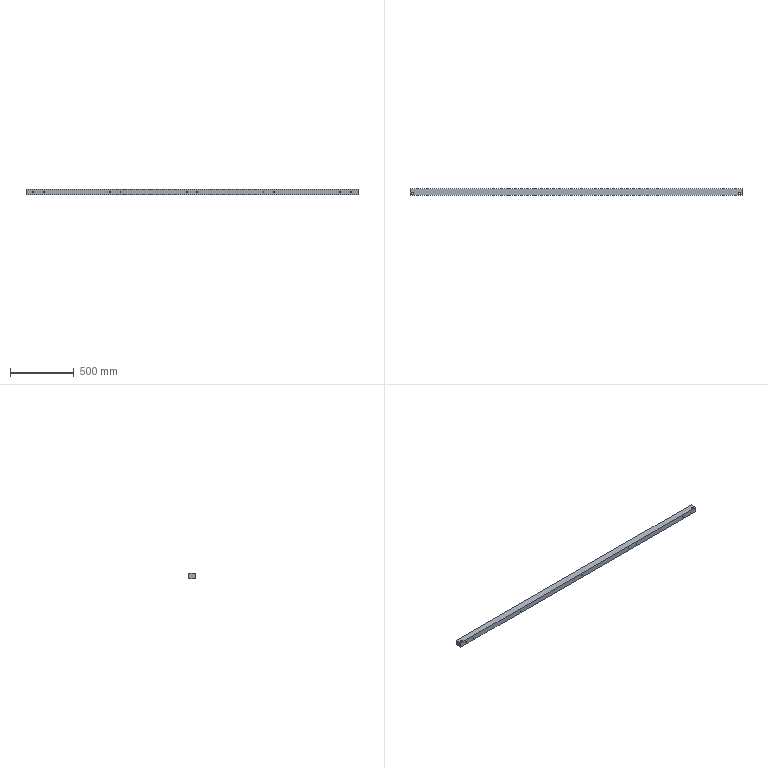Part | SolidWorks | features ICE 2, Extrusion 1 | 1 solid | 30 faces | box 2596 x 50 x 40 mm | volume 5166098 mm3 | cylinder 24 | plane 6 | commonest cylinder face diameters 5 x20 16 x4
STEP:
#1=CARTESIAN_POINT('',(1286.,15.,20.));
#2=VERTEX_POINT('',#1);
#3=CARTESIAN_POINT('',(1270.,15.,20.));
#4=VERTEX_POINT('',#3);
#5=CARTESIAN_POINT('',(1278.,15.,20.));
#6=DIRECTION('',(0.,0.,-1.));
#7=DIRECTION('',(-1.,0.,0.));
#8=AXIS2_PLACEMENT_3D('',#5,#6,#7);
#9=CIRCLE('',#8,8.);
#10=EDGE_CURVE('',#2,#4,#9,.T.);
#11=ORIENTED_EDGE('',*,*,#10,.F.);
#12=CARTESIAN_POINT('',(1286.,15.,-20.));
#13=VERTEX_POINT('',#12);
#14=CARTESIAN_POINT('',(1286.,15.,30.));
#15=DIRECTION('',(0.,0.,-1.));
#16=VECTOR('',#15,1000.);
#17=LINE('',#14,#16);
#18=EDGE_CURVE('',#2,#13,#17,.T.);
#19=ORIENTED_EDGE('',*,*,#18,.T.);
#20=CARTESIAN_POINT('',(1270.,15.,-20.));
#21=VERTEX_POINT('',#20);
#22=CARTESIAN_POINT('',(1278.,15.,-20.));
#23=DIRECTION('',(0.,0.,-1.));
#24=DIRECTION('',(-1.,0.,0.));
#25=AXIS2_PLACEMENT_3D('',#22,#23,#24);
#26=CIRCLE('',#25,8.);
#27=EDGE_CURVE('',#13,#21,#26,.T.);
#28=ORIENTED_EDGE('',*,*,#27,.T.);
#29=CARTESIAN_POINT('',(1270.,15.,30.));
#30=DIRECTION('',(0.,0.,-1.));
#31=VECTOR('',#30,1000.);
#32=LINE('',#29,#31);
#33=EDGE_CURVE('',#4,#21,#32,.T.);
#34=ORIENTED_EDGE('',*,*,#33,.F.);
#35=EDGE_LOOP('',(#11,#19,#28,#34));
#36=FACE_OUTER_BOUND('',#35,.T.);
#37=CARTESIAN_POINT('',(1278.,15.,30.));
#38=DIRECTION('',(0.,0.,-1.));
#39=DIRECTION('',(-1.,0.,0.));
#40=AXIS2_PLACEMENT_3D('',#37,#38,#39);
#41=CYLINDRICAL_SURFACE('',#40,8.);
#42=ADVANCED_FACE('',(#36),#41,.F.);
#43=CARTESIAN_POINT('',(-1270.,15.,20.));
#44=VERTEX_POINT('',#43);
#45=CARTESIAN_POINT('',(-1286.,15.,20.));
#46=VERTEX_POINT('',#45);
#47=CARTESIAN_POINT('',(-1278.,15.,20.));
#48=DIRECTION('',(0.,0.,-1.));
#49=DIRECTION('',(-1.,0.,0.));
#50=AXIS2_PLACEMENT_3D('',#47,#48,#49);
#51=CIRCLE('',#50,8.);
#52=EDGE_CURVE('',#44,#46,#51,.T.);
#53=ORIENTED_EDGE('',*,*,#52,.F.);
#54=CARTESIAN_POINT('',(-1270.,15.,-20.));
#55=VERTEX_POINT('',#54);
#56=CARTESIAN_POINT('',(-1270.,15.,30.));
#57=DIRECTION('',(0.,0.,-1.));
#58=VECTOR('',#57,1000.);
#59=LINE('',#56,#58);
#60=EDGE_CURVE('',#44,#55,#59,.T.);
#61=ORIENTED_EDGE('',*,*,#60,.T.);
#62=CARTESIAN_POINT('',(-1286.,15.,-20.));
#63=VERTEX_POINT('',#62);
#64=CARTESIAN_POINT('',(-1278.,15.,-20.));
#65=DIRECTION('',(0.,0.,-1.));
#66=DIRECTION('',(1.,0.,0.));
#67=AXIS2_PLACEMENT_3D('',#64,#65,#66);
#68=CIRCLE('',#67,8.);
#69=EDGE_CURVE('',#55,#63,#68,.T.);
#70=ORIENTED_EDGE('',*,*,#69,.T.);
#71=CARTESIAN_POINT('',(-1286.,15.,30.));
#72=DIRECTION('',(0.,0.,-1.));
#73=VECTOR('',#72,1000.);
#74=LINE('',#71,#73);
#75=EDGE_CURVE('',#46,#63,#74,.T.);
#76=ORIENTED_EDGE('',*,*,#75,.F.);
#77=EDGE_LOOP('',(#53,#61,#70,#76));
#78=FACE_OUTER_BOUND('',#77,.T.);
#79=CARTESIAN_POINT('',(-1278.,15.,30.));
#80=DIRECTION('',(0.,0.,-1.));
#81=DIRECTION('',(-1.,0.,0.));
#82=AXIS2_PLACEMENT_3D('',#79,#80,#81);
#83=CYLINDRICAL_SURFACE('',#82,8.);
#84=ADVANCED_FACE('',(#78),#83,.F.);
#85=CARTESIAN_POINT('',(1241.5,50.,2.5));
#86=VERTEX_POINT('',#85);
#87=CARTESIAN_POINT('',(1241.5,50.,-2.5));
#88=VERTEX_POINT('',#87);
#89=CARTESIAN_POINT('',(1241.5,50.,0.));
#90=DIRECTION('',(0.,-1.,0.));
#91=DIRECTION('',(0.,0.,-1.));
#92=AXIS2_PLACEMENT_3D('',#89,#90,#91);
#93=CIRCLE('',#92,2.5);
#94=EDGE_CURVE('',#86,#88,#93,.T.);
#95=ORIENTED_EDGE('',*,*,#94,.F.);
#96=CARTESIAN_POINT('',(1241.5,0.,2.5));
#97=VERTEX_POINT('',#96);
#98=CARTESIAN_POINT('',(1241.5,50.,2.5));
#99=DIRECTION('',(0.,-1.,0.));
#100=VECTOR('',#99,1000.);
#101=LINE('',#98,#100);
#102=EDGE_CURVE('',#86,#97,#101,.T.);
#103=ORIENTED_EDGE('',*,*,#102,.T.);
#104=CARTESIAN_POINT('',(1241.5,0.,-2.5));
#105=VERTEX_POINT('',#104);
#106=CARTESIAN_POINT('',(1241.5,0.,0.));
#107=DIRECTION('',(0.,-1.,0.));
#108=DIRECTION('',(0.,0.,-1.));
#109=AXIS2_PLACEMENT_3D('',#106,#107,#108);
#110=CIRCLE('',#109,2.5);
#111=EDGE_CURVE('',#97,#105,#110,.T.);
#112=ORIENTED_EDGE('',*,*,#111,.T.);
#113=CARTESIAN_POINT('',(1241.5,50.,-2.5));
#114=DIRECTION('',(0.,-1.,0.));
#115=VECTOR('',#114,1000.);
#116=LINE('',#113,#115);
#117=EDGE_CURVE('',#88,#105,#116,.T.);
#118=ORIENTED_EDGE('',*,*,#117,.F.);
#119=EDGE_LOOP('',(#95,#103,#112,#118));
#120=FACE_OUTER_BOUND('',#119,.T.);
#121=CARTESIAN_POINT('',(1241.5,50.,0.));
#122=DIRECTION('',(0.,-1.,0.));
#123=DIRECTION('',(0.,0.,-1.));
#124=AXIS2_PLACEMENT_3D('',#121,#122,#123);
#125=CYLINDRICAL_SURFACE('',#124,2.5);
#126=ADVANCED_FACE('',(#120),#125,.F.);
#127=CARTESIAN_POINT('',(1158.5,50.,2.5));
#128=VERTEX_POINT('',#127);
#129=CARTESIAN_POINT('',(1158.5,50.,-2.5));
#130=VERTEX_POINT('',#129);
#131=CARTESIAN_POINT('',(1158.5,50.,0.));
#132=DIRECTION('',(0.,-1.,0.));
#133=DIRECTION('',(0.,0.,-1.));
#134=AXIS2_PLACEMENT_3D('',#131,#132,#133);
#135=CIRCLE('',#134,2.5);
#136=EDGE_CURVE('',#128,#130,#135,.T.);
#137=ORIENTED_EDGE('',*,*,#136,.F.);
#138=CARTESIAN_POINT('',(1158.5,0.,2.5));
#139=VERTEX_POINT('',#138);
#140=CARTESIAN_POINT('',(1158.5,50.,2.5));
#141=DIRECTION('',(0.,-1.,0.));
#142=VECTOR('',#141,1000.);
#143=LINE('',#140,#142);
#144=EDGE_CURVE('',#128,#139,#143,.T.);
#145=ORIENTED_EDGE('',*,*,#144,.T.);
#146=CARTESIAN_POINT('',(1158.5,0.,-2.5));
#147=VERTEX_POINT('',#146);
#148=CARTESIAN_POINT('',(1158.5,0.,0.));
#149=DIRECTION('',(0.,-1.,0.));
#150=DIRECTION('',(0.,0.,-1.));
#151=AXIS2_PLACEMENT_3D('',#148,#149,#150);
#152=CIRCLE('',#151,2.5);
#153=EDGE_CURVE('',#139,#147,#152,.T.);
#154=ORIENTED_EDGE('',*,*,#153,.T.);
#155=CARTESIAN_POINT('',(1158.5,50.,-2.5));
#156=DIRECTION('',(0.,-1.,0.));
#157=VECTOR('',#156,1000.);
#158=LINE('',#155,#157);
#159=EDGE_CURVE('',#130,#147,#158,.T.);
#160=ORIENTED_EDGE('',*,*,#159,.F.);
#161=EDGE_LOOP('',(#137,#145,#154,#160));
#162=FACE_OUTER_BOUND('',#161,.T.);
#163=CARTESIAN_POINT('',(1158.5,50.,0.));
#164=DIRECTION('',(0.,-1.,0.));
#165=DIRECTION('',(0.,0.,-1.));
#166=AXIS2_PLACEMENT_3D('',#163,#164,#165);
#167=CYLINDRICAL_SURFACE('',#166,2.5);
#168=ADVANCED_FACE('',(#162),#167,.F.);
#169=CARTESIAN_POINT('',(641.5,50.,2.5));
#170=VERTEX_POINT('',#169);
#171=CARTESIAN_POINT('',(641.5,50.,-2.5));
#172=VERTEX_POINT('',#171);
#173=CARTESIAN_POINT('',(641.5,50.,0.));
#174=DIRECTION('',(0.,-1.,0.));
#175=DIRECTION('',(0.,0.,-1.));
#176=AXIS2_PLACEMENT_3D('',#173,#174,#175);
#177=CIRCLE('',#176,2.5);
#178=EDGE_CURVE('',#170,#172,#177,.T.);
#179=ORIENTED_EDGE('',*,*,#178,.F.);
#180=CARTESIAN_POINT('',(641.5,0.,2.5));
#181=VERTEX_POINT('',#180);
#182=CARTESIAN_POINT('',(641.5,50.,2.5));
#183=DIRECTION('',(0.,-1.,0.));
#184=VECTOR('',#183,1000.);
#185=LINE('',#182,#184);
#186=EDGE_CURVE('',#170,#181,#185,.T.);
#187=ORIENTED_EDGE('',*,*,#186,.T.);
#188=CARTESIAN_POINT('',(641.5,0.,-2.5));
#189=VERTEX_POINT('',#188);
#190=CARTESIAN_POINT('',(641.5,0.,0.));
#191=DIRECTION('',(0.,-1.,0.));
#192=DIRECTION('',(0.,0.,-1.));
#193=AXIS2_PLACEMENT_3D('',#190,#191,#192);
#194=CIRCLE('',#193,2.5);
#195=EDGE_CURVE('',#181,#189,#194,.T.);
#196=ORIENTED_EDGE('',*,*,#195,.T.);
#197=CARTESIAN_POINT('',(641.5,50.,-2.5));
#198=DIRECTION('',(0.,-1.,0.));
#199=VECTOR('',#198,1000.);
#200=LINE('',#197,#199);
#201=EDGE_CURVE('',#172,#189,#200,.T.);
#202=ORIENTED_EDGE('',*,*,#201,.F.);
#203=EDGE_LOOP('',(#179,#187,#196,#202));
#204=FACE_OUTER_BOUND('',#203,.T.);
#205=CARTESIAN_POINT('',(641.5,50.,0.));
#206=DIRECTION('',(0.,-1.,0.));
#207=DIRECTION('',(0.,0.,-1.));
#208=AXIS2_PLACEMENT_3D('',#205,#206,#207);
#209=CYLINDRICAL_SURFACE('',#208,2.5);
#210=ADVANCED_FACE('',(#204),#209,.F.);
#211=CARTESIAN_POINT('',(558.5,50.,2.5));
#212=VERTEX_POINT('',#211);
#213=CARTESIAN_POINT('',(558.5,50.,-2.5));
#214=VERTEX_POINT('',#213);
#215=CARTESIAN_POINT('',(558.5,50.,0.));
#216=DIRECTION('',(0.,-1.,0.));
#217=DIRECTION('',(0.,0.,-1.));
#218=AXIS2_PLACEMENT_3D('',#215,#216,#217);
#219=CIRCLE('',#218,2.5);
#220=EDGE_CURVE('',#212,#214,#219,.T.);
#221=ORIENTED_EDGE('',*,*,#220,.F.);
#222=CARTESIAN_POINT('',(558.5,0.,2.5));
#223=VERTEX_POINT('',#222);
#224=CARTESIAN_POINT('',(558.5,50.,2.5));
#225=DIRECTION('',(0.,-1.,0.));
#226=VECTOR('',#225,1000.);
#227=LINE('',#224,#226);
#228=EDGE_CURVE('',#212,#223,#227,.T.);
#229=ORIENTED_EDGE('',*,*,#228,.T.);
#230=CARTESIAN_POINT('',(558.5,0.,-2.5));
#231=VERTEX_POINT('',#230);
#232=CARTESIAN_POINT('',(558.5,0.,0.));
#233=DIRECTION('',(0.,-1.,0.));
#234=DIRECTION('',(0.,0.,-1.));
#235=AXIS2_PLACEMENT_3D('',#232,#233,#234);
#236=CIRCLE('',#235,2.5);
#237=EDGE_CURVE('',#223,#231,#236,.T.);
#238=ORIENTED_EDGE('',*,*,#237,.T.);
#239=CARTESIAN_POINT('',(558.5,50.,-2.5));
#240=DIRECTION('',(0.,-1.,0.));
#241=VECTOR('',#240,1000.);
#242=LINE('',#239,#241);
#243=EDGE_CURVE('',#214,#231,#242,.T.);
#244=ORIENTED_EDGE('',*,*,#243,.F.);
#245=EDGE_LOOP('',(#221,#229,#238,#244));
#246=FACE_OUTER_BOUND('',#245,.T.);
#247=CARTESIAN_POINT('',(558.5,50.,0.));
#248=DIRECTION('',(0.,-1.,0.));
#249=DIRECTION('',(0.,0.,-1.));
#250=AXIS2_PLACEMENT_3D('',#247,#248,#249);
#251=CYLINDRICAL_SURFACE('',#250,2.5);
#252=ADVANCED_FACE('',(#246),#251,.F.);
#253=CARTESIAN_POINT('',(41.5,50.,2.5));
#254=VERTEX_POINT('',#253);
#255=CARTESIAN_POINT('',(41.5,50.,-2.5));
#256=VERTEX_POINT('',#255);
#257=CARTESIAN_POINT('',(41.5,50.,0.));
#258=DIRECTION('',(0.,-1.,0.));
#259=DIRECTION('',(0.,0.,-1.));
#260=AXIS2_PLACEMENT_3D('',#257,#258,#259);
#261=CIRCLE('',#260,2.5);
#262=EDGE_CURVE('',#254,#256,#261,.T.);
#263=ORIENTED_EDGE('',*,*,#262,.F.);
#264=CARTESIAN_POINT('',(41.5,0.,2.5));
#265=VERTEX_POINT('',#264);
#266=CARTESIAN_POINT('',(41.5,50.,2.5));
#267=DIRECTION('',(0.,-1.,0.));
#268=VECTOR('',#267,1000.);
#269=LINE('',#266,#268);
#270=EDGE_CURVE('',#254,#265,#269,.T.);
#271=ORIENTED_EDGE('',*,*,#270,.T.);
#272=CARTESIAN_POINT('',(41.5,0.,-2.5));
#273=VERTEX_POINT('',#272);
#274=CARTESIAN_POINT('',(41.5,0.,0.));
#275=DIRECTION('',(0.,-1.,0.));
#276=DIRECTION('',(0.,0.,-1.));
#277=AXIS2_PLACEMENT_3D('',#274,#275,#276);
#278=CIRCLE('',#277,2.5);
#279=EDGE_CURVE('',#265,#273,#278,.T.);
#280=ORIENTED_EDGE('',*,*,#279,.T.);
#281=CARTESIAN_POINT('',(41.5,50.,-2.5));
#282=DIRECTION('',(0.,-1.,0.));
#283=VECTOR('',#282,1000.);
#284=LINE('',#281,#283);
#285=EDGE_CURVE('',#256,#273,#284,.T.);
#286=ORIENTED_EDGE('',*,*,#285,.F.);
#287=EDGE_LOOP('',(#263,#271,#280,#286));
#288=FACE_OUTER_BOUND('',#287,.T.);
#289=CARTESIAN_POINT('',(41.5,50.,0.));
#290=DIRECTION('',(0.,-1.,0.));
#291=DIRECTION('',(0.,0.,-1.));
#292=AXIS2_PLACEMENT_3D('',#289,#290,#291);
#293=CYLINDRICAL_SURFACE('',#292,2.5);
#294=ADVANCED_FACE('',(#288),#293,.F.);
#295=CARTESIAN_POINT('',(-41.5,50.,2.5));
#296=VERTEX_POINT('',#295);
#297=CARTESIAN_POINT('',(-41.5,50.,-2.5));
#298=VERTEX_POINT('',#297);
#299=CARTESIAN_POINT('',(-41.5,50.,0.));
#300=DIRECTION('',(0.,-1.,0.));
#301=DIRECTION('',(0.,0.,1.));
#302=AXIS2_PLACEMENT_3D('',#299,#300,#301);
#303=CIRCLE('',#302,2.5);
#304=EDGE_CURVE('',#296,#298,#303,.T.);
#305=ORIENTED_EDGE('',*,*,#304,.F.);
#306=CARTESIAN_POINT('',(-41.5,0.,2.5));
#307=VERTEX_POINT('',#306);
#308=CARTESIAN_POINT('',(-41.5,50.,2.5));
#309=DIRECTION('',(0.,-1.,0.));
#310=VECTOR('',#309,1000.);
#311=LINE('',#308,#310);
#312=EDGE_CURVE('',#296,#307,#311,.T.);
#313=ORIENTED_EDGE('',*,*,#312,.T.);
#314=CARTESIAN_POINT('',(-41.5,0.,-2.5));
#315=VERTEX_POINT('',#314);
#316=CARTESIAN_POINT('',(-41.5,0.,0.));
#317=DIRECTION('',(0.,-1.,0.));
#318=DIRECTION('',(0.,0.,1.));
#319=AXIS2_PLACEMENT_3D('',#316,#317,#318);
#320=CIRCLE('',#319,2.5);
#321=EDGE_CURVE('',#307,#315,#320,.T.);
#322=ORIENTED_EDGE('',*,*,#321,.T.);
#323=CARTESIAN_POINT('',(-41.5,50.,-2.5));
#324=DIRECTION('',(0.,-1.,0.));
#325=VECTOR('',#324,1000.);
#326=LINE('',#323,#325);
#327=EDGE_CURVE('',#298,#315,#326,.T.);
#328=ORIENTED_EDGE('',*,*,#327,.F.);
#329=EDGE_LOOP('',(#305,#313,#322,#328));
#330=FACE_OUTER_BOUND('',#329,.T.);
#331=CARTESIAN_POINT('',(-41.5,50.,0.));
#332=DIRECTION('',(0.,-1.,0.));
#333=DIRECTION('',(0.,0.,-1.));
#334=AXIS2_PLACEMENT_3D('',#331,#332,#333);
#335=CYLINDRICAL_SURFACE('',#334,2.5);
#336=ADVANCED_FACE('',(#330),#335,.F.);
#337=CARTESIAN_POINT('',(-558.5,50.,2.5));
#338=VERTEX_POINT('',#337);
#339=CARTESIAN_POINT('',(-558.5,50.,-2.5));
#340=VERTEX_POINT('',#339);
#341=CARTESIAN_POINT('',(-558.5,50.,0.));
#342=DIRECTION('',(0.,-1.,0.));
#343=DIRECTION('',(0.,0.,1.));
#344=AXIS2_PLACEMENT_3D('',#341,#342,#343);
#345=CIRCLE('',#344,2.5);
#346=EDGE_CURVE('',#338,#340,#345,.T.);
#347=ORIENTED_EDGE('',*,*,#346,.F.);
#348=CARTESIAN_POINT('',(-558.5,0.,2.5));
#349=VERTEX_POINT('',#348);
#350=CARTESIAN_POINT('',(-558.5,50.,2.5));
#351=DIRECTION('',(0.,-1.,0.));
#352=VECTOR('',#351,1000.);
#353=LINE('',#350,#352);
#354=EDGE_CURVE('',#338,#349,#353,.T.);
#355=ORIENTED_EDGE('',*,*,#354,.T.);
#356=CARTESIAN_POINT('',(-558.5,0.,-2.5));
#357=VERTEX_POINT('',#356);
#358=CARTESIAN_POINT('',(-558.5,0.,0.));
#359=DIRECTION('',(0.,-1.,0.));
#360=DIRECTION('',(0.,0.,1.));
#361=AXIS2_PLACEMENT_3D('',#358,#359,#360);
#362=CIRCLE('',#361,2.5);
#363=EDGE_CURVE('',#349,#357,#362,.T.);
#364=ORIENTED_EDGE('',*,*,#363,.T.);
#365=CARTESIAN_POINT('',(-558.5,50.,-2.5));
#366=DIRECTION('',(0.,-1.,0.));
#367=VECTOR('',#366,1000.);
#368=LINE('',#365,#367);
#369=EDGE_CURVE('',#340,#357,#368,.T.);
#370=ORIENTED_EDGE('',*,*,#369,.F.);
#371=EDGE_LOOP('',(#347,#355,#364,#370));
#372=FACE_OUTER_BOUND('',#371,.T.);
#373=CARTESIAN_POINT('',(-558.5,50.,0.));
#374=DIRECTION('',(0.,-1.,0.));
#375=DIRECTION('',(0.,0.,-1.));
#376=AXIS2_PLACEMENT_3D('',#373,#374,#375);
#377=CYLINDRICAL_SURFACE('',#376,2.5);
#378=ADVANCED_FACE('',(#372),#377,.F.);
#379=CARTESIAN_POINT('',(-641.5,50.,2.5));
#380=VERTEX_POINT('',#379);
#381=CARTESIAN_POINT('',(-641.5,50.,-2.5));
#382=VERTEX_POINT('',#381);
#383=CARTESIAN_POINT('',(-641.5,50.,0.));
#384=DIRECTION('',(0.,-1.,0.));
#385=DIRECTION('',(0.,0.,1.));
#386=AXIS2_PLACEMENT_3D('',#383,#384,#385);
#387=CIRCLE('',#386,2.5);
#388=EDGE_CURVE('',#380,#382,#387,.T.);
#389=ORIENTED_EDGE('',*,*,#388,.F.);
#390=CARTESIAN_POINT('',(-641.5,0.,2.5));
#391=VERTEX_POINT('',#390);
#392=CARTESIAN_POINT('',(-641.5,50.,2.5));
#393=DIRECTION('',(0.,-1.,0.));
#394=VECTOR('',#393,1000.);
#395=LINE('',#392,#394);
#396=EDGE_CURVE('',#380,#391,#395,.T.);
#397=ORIENTED_EDGE('',*,*,#396,.T.);
#398=CARTESIAN_POINT('',(-641.5,0.,-2.5));
#399=VERTEX_POINT('',#398);
#400=CARTESIAN_POINT('',(-641.5,0.,0.));
#401=DIRECTION('',(0.,-1.,0.));
#402=DIRECTION('',(0.,0.,1.));
#403=AXIS2_PLACEMENT_3D('',#400,#401,#402);
#404=CIRCLE('',#403,2.5);
#405=EDGE_CURVE('',#391,#399,#404,.T.);
#406=ORIENTED_EDGE('',*,*,#405,.T.);
#407=CARTESIAN_POINT('',(-641.5,50.,-2.5));
#408=DIRECTION('',(0.,-1.,0.));
#409=VECTOR('',#408,1000.);
#410=LINE('',#407,#409);
#411=EDGE_CURVE('',#382,#399,#410,.T.);
#412=ORIENTED_EDGE('',*,*,#411,.F.);
#413=EDGE_LOOP('',(#389,#397,#406,#412));
#414=FACE_OUTER_BOUND('',#413,.T.);
#415=CARTESIAN_POINT('',(-641.5,50.,0.));
#416=DIRECTION('',(0.,-1.,0.));
#417=DIRECTION('',(0.,0.,-1.));
#418=AXIS2_PLACEMENT_3D('',#415,#416,#417);
#419=CYLINDRICAL_SURFACE('',#418,2.5);
#420=ADVANCED_FACE('',(#414),#419,.F.);
#421=CARTESIAN_POINT('',(-1158.5,50.,2.5));
#422=VERTEX_POINT('',#421);
#423=CARTESIAN_POINT('',(-1158.5,50.,-2.5));
#424=VERTEX_POINT('',#423);
#425=CARTESIAN_POINT('',(-1158.5,50.,0.));
#426=DIRECTION('',(0.,-1.,0.));
#427=DIRECTION('',(0.,0.,1.));
#428=AXIS2_PLACEMENT_3D('',#425,#426,#427);
#429=CIRCLE('',#428,2.5);
#430=EDGE_CURVE('',#422,#424,#429,.T.);
#431=ORIENTED_EDGE('',*,*,#430,.F.);
#432=CARTESIAN_POINT('',(-1158.5,0.,2.5));
#433=VERTEX_POINT('',#432);
#434=CARTESIAN_POINT('',(-1158.5,50.,2.5));
#435=DIRECTION('',(0.,-1.,0.));
#436=VECTOR('',#435,1000.);
#437=LINE('',#434,#436);
#438=EDGE_CURVE('',#422,#433,#437,.T.);
#439=ORIENTED_EDGE('',*,*,#438,.T.);
#440=CARTESIAN_POINT('',(-1158.5,0.,-2.5));
#441=VERTEX_POINT('',#440);
#442=CARTESIAN_POINT('',(-1158.5,0.,0.));
#443=DIRECTION('',(0.,-1.,0.));
#444=DIRECTION('',(0.,0.,1.));
#445=AXIS2_PLACEMENT_3D('',#442,#443,#444);
#446=CIRCLE('',#445,2.5);
#447=EDGE_CURVE('',#433,#441,#446,.T.);
#448=ORIENTED_EDGE('',*,*,#447,.T.);
#449=CARTESIAN_POINT('',(-1158.5,50.,-2.5));
#450=DIRECTION('',(0.,-1.,0.));
#451=VECTOR('',#450,1000.);
#452=LINE('',#449,#451);
#453=EDGE_CURVE('',#424,#441,#452,.T.);
#454=ORIENTED_EDGE('',*,*,#453,.F.);
#455=EDGE_LOOP('',(#431,#439,#448,#454));
#456=FACE_OUTER_BOUND('',#455,.T.);
#457=CARTESIAN_POINT('',(-1158.5,50.,0.));
#458=DIRECTION('',(0.,-1.,0.));
#459=DIRECTION('',(0.,0.,-1.));
#460=AXIS2_PLACEMENT_3D('',#457,#458,#459);
#461=CYLINDRICAL_SURFACE('',#460,2.5);
#462=ADVANCED_FACE('',(#456),#461,.F.);
#463=CARTESIAN_POINT('',(-1241.5,50.,2.5));
#464=VERTEX_POINT('',#463);
#465=CARTESIAN_POINT('',(-1241.5,50.,-2.5));
#466=VERTEX_POINT('',#465);
#467=CARTESIAN_POINT('',(-1241.5,50.,0.));
#468=DIRECTION('',(0.,-1.,0.));
#469=DIRECTION('',(0.,0.,1.));
#470=AXIS2_PLACEMENT_3D('',#467,#468,#469);
#471=CIRCLE('',#470,2.5);
#472=EDGE_CURVE('',#464,#466,#471,.T.);
#473=ORIENTED_EDGE('',*,*,#472,.F.);
#474=CARTESIAN_POINT('',(-1241.5,0.,2.5));
#475=VERTEX_POINT('',#474);
#476=CARTESIAN_POINT('',(-1241.5,50.,2.5));
#477=DIRECTION('',(0.,-1.,0.));
#478=VECTOR('',#477,1000.);
#479=LINE('',#476,#478);
#480=EDGE_CURVE('',#464,#475,#479,.T.);
#481=ORIENTED_EDGE('',*,*,#480,.T.);
#482=CARTESIAN_POINT('',(-1241.5,0.,-2.5));
#483=VERTEX_POINT('',#482);
#484=CARTESIAN_POINT('',(-1241.5,0.,0.));
#485=DIRECTION('',(0.,-1.,0.));
#486=DIRECTION('',(0.,0.,1.));
#487=AXIS2_PLACEMENT_3D('',#484,#485,#486);
#488=CIRCLE('',#487,2.5);
#489=EDGE_CURVE('',#475,#483,#488,.T.);
#490=ORIENTED_EDGE('',*,*,#489,.T.);
#491=CARTESIAN_POINT('',(-1241.5,50.,-2.5));
#492=DIRECTION('',(0.,-1.,0.));
#493=VECTOR('',#492,1000.);
#494=LINE('',#491,#493);
#495=EDGE_CURVE('',#466,#483,#494,.T.);
#496=ORIENTED_EDGE('',*,*,#495,.F.);
#497=EDGE_LOOP('',(#473,#481,#490,#496));
#498=FACE_OUTER_BOUND('',#497,.T.);
#499=CARTESIAN_POINT('',(-1241.5,50.,0.));
#500=DIRECTION('',(0.,-1.,0.));
#501=DIRECTION('',(0.,0.,-1.));
#502=AXIS2_PLACEMENT_3D('',#499,#500,#501);
#503=CYLINDRICAL_SURFACE('',#502,2.5);
#504=ADVANCED_FACE('',(#498),#503,.F.);
#505=CARTESIAN_POINT('',(1298.,0.,20.));
#506=VERTEX_POINT('',#505);
#507=CARTESIAN_POINT('',(1298.,0.,-20.));
#508=VERTEX_POINT('',#507);
#509=CARTESIAN_POINT('',(1298.,0.,20.));
#510=DIRECTION('',(0.,0.,-1.));
#511=VECTOR('',#510,1000.);
#512=LINE('',#509,#511);
#513=EDGE_CURVE('',#506,#508,#512,.T.);
#514=ORIENTED_EDGE('',*,*,#513,.T.);
#515=CARTESIAN_POINT('',(1298.,50.,-20.));
#516=VERTEX_POINT('',#515);
#517=CARTESIAN_POINT('',(1298.,50.,-20.));
#518=DIRECTION('',(0.,-1.,0.));
#519=VECTOR('',#518,1000.);
#520=LINE('',#517,#519);
#521=EDGE_CURVE('',#516,#508,#520,.T.);
#522=ORIENTED_EDGE('',*,*,#521,.F.);
#523=CARTESIAN_POINT('',(1298.,50.,20.));
#524=VERTEX_POINT('',#523);
#525=CARTESIAN_POINT('',(1298.,50.,20.));
#526=DIRECTION('',(0.,0.,-1.));
#527=VECTOR('',#526,1000.);
#528=LINE('',#525,#527);
#529=EDGE_CURVE('',#524,#516,#528,.T.);
#530=ORIENTED_EDGE('',*,*,#529,.F.);
#531=CARTESIAN_POINT('',(1298.,50.,20.));
#532=DIRECTION('',(0.,-1.,0.));
#533=VECTOR('',#532,1000.);
#534=LINE('',#531,#533);
#535=EDGE_CURVE('',#524,#506,#534,.T.);
#536=ORIENTED_EDGE('',*,*,#535,.T.);
#537=EDGE_LOOP('',(#514,#522,#530,#536));
#538=FACE_OUTER_BOUND('',#537,.T.);
#539=CARTESIAN_POINT('',(1298.,50.,20.));
#540=DIRECTION('',(-1.,0.,0.));
#541=DIRECTION('',(0.,0.,1.));
#542=AXIS2_PLACEMENT_3D('',#539,#540,#541);
#543=PLANE('',#542);
#544=ADVANCED_FACE('',(#538),#543,.F.);
#545=CARTESIAN_POINT('',(1278.,15.,-20.));
#546=DIRECTION('',(0.,0.,-1.));
#547=DIRECTION('',(-1.,0.,0.));
#548=AXIS2_PLACEMENT_3D('',#545,#546,#547);
#549=CIRCLE('',#548,8.);
#550=EDGE_CURVE('',#21,#13,#549,.T.);
#551=ORIENTED_EDGE('',*,*,#550,.F.);
#552=ORIENTED_EDGE('',*,*,#27,.F.);
#553=EDGE_LOOP('',(#551,#552));
#554=FACE_BOUND('',#553,.T.);
#555=CARTESIAN_POINT('',(-1278.,15.,-20.));
#556=DIRECTION('',(0.,0.,-1.));
#557=DIRECTION('',(1.,0.,0.));
#558=AXIS2_PLACEMENT_3D('',#555,#556,#557);
#559=CIRCLE('',#558,8.);
#560=EDGE_CURVE('',#63,#55,#559,.T.);
#561=ORIENTED_EDGE('',*,*,#560,.F.);
#562=ORIENTED_EDGE('',*,*,#69,.F.);
#563=EDGE_LOOP('',(#561,#562));
#564=FACE_BOUND('',#563,.T.);
#565=CARTESIAN_POINT('',(-1298.,0.,-20.));
#566=VERTEX_POINT('',#565);
#567=CARTESIAN_POINT('',(-1298.,0.,-20.));
#568=DIRECTION('',(-1.,0.,0.));
#569=VECTOR('',#568,1000.);
#570=LINE('',#567,#569);
#571=EDGE_CURVE('',#508,#566,#570,.T.);
#572=ORIENTED_EDGE('',*,*,#571,.T.);
#573=CARTESIAN_POINT('',(-1298.,50.,-20.));
#574=VERTEX_POINT('',#573);
#575=CARTESIAN_POINT('',(-1298.,50.,-20.));
#576=DIRECTION('',(0.,-1.,0.));
#577=VECTOR('',#576,1000.);
#578=LINE('',#575,#577);
#579=EDGE_CURVE('',#574,#566,#578,.T.);
#580=ORIENTED_EDGE('',*,*,#579,.F.);
#581=CARTESIAN_POINT('',(-1298.,50.,-20.));
#582=DIRECTION('',(-1.,0.,0.));
#583=VECTOR('',#582,1000.);
#584=LINE('',#581,#583);
#585=EDGE_CURVE('',#516,#574,#584,.T.);
#586=ORIENTED_EDGE('',*,*,#585,.F.);
#587=ORIENTED_EDGE('',*,*,#521,.T.);
#588=EDGE_LOOP('',(#572,#580,#586,#587));
#589=FACE_OUTER_BOUND('',#588,.T.);
#590=CARTESIAN_POINT('',(-1298.,50.,-20.));
#591=DIRECTION('',(0.,0.,1.));
#592=DIRECTION('',(1.,0.,0.));
#593=AXIS2_PLACEMENT_3D('',#590,#591,#592);
#594=PLANE('',#593);
#595=ADVANCED_FACE('',(#554,#564,#589),#594,.F.);
#596=CARTESIAN_POINT('',(-1298.,0.,20.));
#597=VERTEX_POINT('',#596);
#598=CARTESIAN_POINT('',(-1298.,0.,20.));
#599=DIRECTION('',(0.,0.,1.));
#600=VECTOR('',#599,1000.);
#601=LINE('',#598,#600);
#602=EDGE_CURVE('',#566,#597,#601,.T.);
#603=ORIENTED_EDGE('',*,*,#602,.T.);
#604=CARTESIAN_POINT('',(-1298.,50.,20.));
#605=VERTEX_POINT('',#604);
#606=CARTESIAN_POINT('',(-1298.,50.,20.));
#607=DIRECTION('',(0.,-1.,0.));
#608=VECTOR('',#607,1000.);
#609=LINE('',#606,#608);
#610=EDGE_CURVE('',#605,#597,#609,.T.);
#611=ORIENTED_EDGE('',*,*,#610,.F.);
#612=CARTESIAN_POINT('',(-1298.,50.,20.));
#613=DIRECTION('',(0.,0.,1.));
#614=VECTOR('',#613,1000.);
#615=LINE('',#612,#614);
#616=EDGE_CURVE('',#574,#605,#615,.T.);
#617=ORIENTED_EDGE('',*,*,#616,.F.);
#618=ORIENTED_EDGE('',*,*,#579,.T.);
#619=EDGE_LOOP('',(#603,#611,#617,#618));
#620=FACE_OUTER_BOUND('',#619,.T.);
#621=CARTESIAN_POINT('',(-1298.,50.,20.));
#622=DIRECTION('',(1.,0.,0.));
#623=DIRECTION('',(0.,0.,-1.));
#624=AXIS2_PLACEMENT_3D('',#621,#622,#623);
#625=PLANE('',#624);
#626=ADVANCED_FACE('',(#620),#625,.F.);
#627=CARTESIAN_POINT('',(1278.,15.,20.));
#628=DIRECTION('',(0.,0.,-1.));
#629=DIRECTION('',(-1.,0.,0.));
#630=AXIS2_PLACEMENT_3D('',#627,#628,#629);
#631=CIRCLE('',#630,8.);
#632=EDGE_CURVE('',#4,#2,#631,.T.);
#633=ORIENTED_EDGE('',*,*,#632,.T.);
#634=ORIENTED_EDGE('',*,*,#10,.T.);
#635=EDGE_LOOP('',(#633,#634));
#636=FACE_BOUND('',#635,.T.);
#637=CARTESIAN_POINT('',(-1278.,15.,20.));
#638=DIRECTION('',(0.,0.,-1.));
#639=DIRECTION('',(-1.,0.,0.));
#640=AXIS2_PLACEMENT_3D('',#637,#638,#639);
#641=CIRCLE('',#640,8.);
#642=EDGE_CURVE('',#46,#44,#641,.T.);
#643=ORIENTED_EDGE('',*,*,#642,.T.);
#644=ORIENTED_EDGE('',*,*,#52,.T.);
#645=EDGE_LOOP('',(#643,#644));
#646=FACE_BOUND('',#645,.T.);
#647=CARTESIAN_POINT('',(-1298.,0.,20.));
#648=DIRECTION('',(1.,0.,0.));
#649=VECTOR('',#648,1000.);
#650=LINE('',#647,#649);
#651=EDGE_CURVE('',#597,#506,#650,.T.);
#652=ORIENTED_EDGE('',*,*,#651,.T.);
#653=ORIENTED_EDGE('',*,*,#535,.F.);
#654=CARTESIAN_POINT('',(-1298.,50.,20.));
#655=DIRECTION('',(1.,0.,0.));
#656=VECTOR('',#655,1000.);
#657=LINE('',#654,#656);
#658=EDGE_CURVE('',#605,#524,#657,.T.);
#659=ORIENTED_EDGE('',*,*,#658,.F.);
#660=ORIENTED_EDGE('',*,*,#610,.T.);
#661=EDGE_LOOP('',(#652,#653,#659,#660));
#662=FACE_OUTER_BOUND('',#661,.T.);
#663=CARTESIAN_POINT('',(-1298.,50.,20.));
#664=DIRECTION('',(0.,0.,-1.));
#665=DIRECTION('',(-1.,0.,0.));
#666=AXIS2_PLACEMENT_3D('',#663,#664,#665);
#667=PLANE('',#666);
#668=ADVANCED_FACE('',(#636,#646,#662),#667,.F.);
#669=CARTESIAN_POINT('',(1241.5,50.,0.));
#670=DIRECTION('',(0.,-1.,0.));
#671=DIRECTION('',(0.,0.,-1.));
#672=AXIS2_PLACEMENT_3D('',#669,#670,#671);
#673=CIRCLE('',#672,2.5);
#674=EDGE_CURVE('',#88,#86,#673,.T.);
#675=ORIENTED_EDGE('',*,*,#674,.T.);
#676=ORIENTED_EDGE('',*,*,#94,.T.);
#677=EDGE_LOOP('',(#675,#676));
#678=FACE_BOUND('',#677,.T.);
#679=CARTESIAN_POINT('',(1158.5,50.,0.));
#680=DIRECTION('',(0.,-1.,0.));
#681=DIRECTION('',(0.,0.,-1.));
#682=AXIS2_PLACEMENT_3D('',#679,#680,#681);
#683=CIRCLE('',#682,2.5);
#684=EDGE_CURVE('',#130,#128,#683,.T.);
#685=ORIENTED_EDGE('',*,*,#684,.T.);
#686=ORIENTED_EDGE('',*,*,#136,.T.);
#687=EDGE_LOOP('',(#685,#686));
#688=FACE_BOUND('',#687,.T.);
#689=CARTESIAN_POINT('',(641.5,50.,0.));
#690=DIRECTION('',(0.,-1.,0.));
#691=DIRECTION('',(0.,0.,-1.));
#692=AXIS2_PLACEMENT_3D('',#689,#690,#691);
#693=CIRCLE('',#692,2.5);
#694=EDGE_CURVE('',#172,#170,#693,.T.);
#695=ORIENTED_EDGE('',*,*,#694,.T.);
#696=ORIENTED_EDGE('',*,*,#178,.T.);
#697=EDGE_LOOP('',(#695,#696));
#698=FACE_BOUND('',#697,.T.);
#699=CARTESIAN_POINT('',(558.5,50.,0.));
#700=DIRECTION('',(0.,-1.,0.));
#701=DIRECTION('',(0.,0.,-1.));
#702=AXIS2_PLACEMENT_3D('',#699,#700,#701);
#703=CIRCLE('',#702,2.5);
#704=EDGE_CURVE('',#214,#212,#703,.T.);
#705=ORIENTED_EDGE('',*,*,#704,.T.);
#706=ORIENTED_EDGE('',*,*,#220,.T.);
#707=EDGE_LOOP('',(#705,#706));
#708=FACE_BOUND('',#707,.T.);
#709=CARTESIAN_POINT('',(41.5,50.,0.));
#710=DIRECTION('',(0.,-1.,0.));
#711=DIRECTION('',(0.,0.,-1.));
#712=AXIS2_PLACEMENT_3D('',#709,#710,#711);
#713=CIRCLE('',#712,2.5);
#714=EDGE_CURVE('',#256,#254,#713,.T.);
#715=ORIENTED_EDGE('',*,*,#714,.T.);
#716=ORIENTED_EDGE('',*,*,#262,.T.);
#717=EDGE_LOOP('',(#715,#716));
#718=FACE_BOUND('',#717,.T.);
#719=CARTESIAN_POINT('',(-41.5,50.,0.));
#720=DIRECTION('',(0.,-1.,0.));
#721=DIRECTION('',(0.,0.,1.));
#722=AXIS2_PLACEMENT_3D('',#719,#720,#721);
#723=CIRCLE('',#722,2.5);
#724=EDGE_CURVE('',#298,#296,#723,.T.);
#725=ORIENTED_EDGE('',*,*,#724,.T.);
#726=ORIENTED_EDGE('',*,*,#304,.T.);
#727=EDGE_LOOP('',(#725,#726));
#728=FACE_BOUND('',#727,.T.);
#729=CARTESIAN_POINT('',(-558.5,50.,0.));
#730=DIRECTION('',(0.,-1.,0.));
#731=DIRECTION('',(0.,0.,1.));
#732=AXIS2_PLACEMENT_3D('',#729,#730,#731);
#733=CIRCLE('',#732,2.5);
#734=EDGE_CURVE('',#340,#338,#733,.T.);
#735=ORIENTED_EDGE('',*,*,#734,.T.);
#736=ORIENTED_EDGE('',*,*,#346,.T.);
#737=EDGE_LOOP('',(#735,#736));
#738=FACE_BOUND('',#737,.T.);
#739=CARTESIAN_POINT('',(-641.5,50.,0.));
#740=DIRECTION('',(0.,-1.,0.));
#741=DIRECTION('',(0.,0.,1.));
#742=AXIS2_PLACEMENT_3D('',#739,#740,#741);
#743=CIRCLE('',#742,2.5);
#744=EDGE_CURVE('',#382,#380,#743,.T.);
#745=ORIENTED_EDGE('',*,*,#744,.T.);
#746=ORIENTED_EDGE('',*,*,#388,.T.);
#747=EDGE_LOOP('',(#745,#746));
#748=FACE_BOUND('',#747,.T.);
#749=CARTESIAN_POINT('',(-1158.5,50.,0.));
#750=DIRECTION('',(0.,-1.,0.));
#751=DIRECTION('',(0.,0.,1.));
#752=AXIS2_PLACEMENT_3D('',#749,#750,#751);
#753=CIRCLE('',#752,2.5);
#754=EDGE_CURVE('',#424,#422,#753,.T.);
#755=ORIENTED_EDGE('',*,*,#754,.T.);
#756=ORIENTED_EDGE('',*,*,#430,.T.);
#757=EDGE_LOOP('',(#755,#756));
#758=FACE_BOUND('',#757,.T.);
#759=CARTESIAN_POINT('',(-1241.5,50.,0.));
#760=DIRECTION('',(0.,-1.,0.));
#761=DIRECTION('',(0.,0.,1.));
#762=AXIS2_PLACEMENT_3D('',#759,#760,#761);
#763=CIRCLE('',#762,2.5);
#764=EDGE_CURVE('',#466,#464,#763,.T.);
#765=ORIENTED_EDGE('',*,*,#764,.T.);
#766=ORIENTED_EDGE('',*,*,#472,.T.);
#767=EDGE_LOOP('',(#765,#766));
#768=FACE_BOUND('',#767,.T.);
#769=ORIENTED_EDGE('',*,*,#529,.T.);
#770=ORIENTED_EDGE('',*,*,#585,.T.);
#771=ORIENTED_EDGE('',*,*,#616,.T.);
#772=ORIENTED_EDGE('',*,*,#658,.T.);
#773=EDGE_LOOP('',(#769,#770,#771,#772));
#774=FACE_OUTER_BOUND('',#773,.T.);
#775=CARTESIAN_POINT('',(0.,50.,0.));
#776=DIRECTION('',(0.,-1.,0.));
#777=DIRECTION('',(0.,0.,-1.));
#778=AXIS2_PLACEMENT_3D('',#775,#776,#777);
#779=PLANE('',#778);
#780=ADVANCED_FACE('',(#678,#688,#698,#708,#718,#728,#738,#748,#758,#768,#774),#779,.F.);
#781=CARTESIAN_POINT('',(1241.5,0.,0.));
#782=DIRECTION('',(0.,-1.,0.));
#783=DIRECTION('',(0.,0.,-1.));
#784=AXIS2_PLACEMENT_3D('',#781,#782,#783);
#785=CIRCLE('',#784,2.5);
#786=EDGE_CURVE('',#105,#97,#785,.T.);
#787=ORIENTED_EDGE('',*,*,#786,.F.);
#788=ORIENTED_EDGE('',*,*,#111,.F.);
#789=EDGE_LOOP('',(#787,#788));
#790=FACE_BOUND('',#789,.T.);
#791=CARTESIAN_POINT('',(1158.5,0.,0.));
#792=DIRECTION('',(0.,-1.,0.));
#793=DIRECTION('',(0.,0.,-1.));
#794=AXIS2_PLACEMENT_3D('',#791,#792,#793);
#795=CIRCLE('',#794,2.5);
#796=EDGE_CURVE('',#147,#139,#795,.T.);
#797=ORIENTED_EDGE('',*,*,#796,.F.);
#798=ORIENTED_EDGE('',*,*,#153,.F.);
#799=EDGE_LOOP('',(#797,#798));
#800=FACE_BOUND('',#799,.T.);
#801=CARTESIAN_POINT('',(641.5,0.,0.));
#802=DIRECTION('',(0.,-1.,0.));
#803=DIRECTION('',(0.,0.,-1.));
#804=AXIS2_PLACEMENT_3D('',#801,#802,#803);
#805=CIRCLE('',#804,2.5);
#806=EDGE_CURVE('',#189,#181,#805,.T.);
#807=ORIENTED_EDGE('',*,*,#806,.F.);
#808=ORIENTED_EDGE('',*,*,#195,.F.);
#809=EDGE_LOOP('',(#807,#808));
#810=FACE_BOUND('',#809,.T.);
#811=CARTESIAN_POINT('',(558.5,0.,0.));
#812=DIRECTION('',(0.,-1.,0.));
#813=DIRECTION('',(0.,0.,-1.));
#814=AXIS2_PLACEMENT_3D('',#811,#812,#813);
#815=CIRCLE('',#814,2.5);
#816=EDGE_CURVE('',#231,#223,#815,.T.);
#817=ORIENTED_EDGE('',*,*,#816,.F.);
#818=ORIENTED_EDGE('',*,*,#237,.F.);
#819=EDGE_LOOP('',(#817,#818));
#820=FACE_BOUND('',#819,.T.);
#821=CARTESIAN_POINT('',(41.5,0.,0.));
#822=DIRECTION('',(0.,-1.,0.));
#823=DIRECTION('',(0.,0.,-1.));
#824=AXIS2_PLACEMENT_3D('',#821,#822,#823);
#825=CIRCLE('',#824,2.5);
#826=EDGE_CURVE('',#273,#265,#825,.T.);
#827=ORIENTED_EDGE('',*,*,#826,.F.);
#828=ORIENTED_EDGE('',*,*,#279,.F.);
#829=EDGE_LOOP('',(#827,#828));
#830=FACE_BOUND('',#829,.T.);
#831=CARTESIAN_POINT('',(-41.5,0.,0.));
#832=DIRECTION('',(0.,-1.,0.));
#833=DIRECTION('',(0.,0.,1.));
#834=AXIS2_PLACEMENT_3D('',#831,#832,#833);
#835=CIRCLE('',#834,2.5);
#836=EDGE_CURVE('',#315,#307,#835,.T.);
#837=ORIENTED_EDGE('',*,*,#836,.F.);
#838=ORIENTED_EDGE('',*,*,#321,.F.);
#839=EDGE_LOOP('',(#837,#838));
#840=FACE_BOUND('',#839,.T.);
#841=CARTESIAN_POINT('',(-558.5,0.,0.));
#842=DIRECTION('',(0.,-1.,0.));
#843=DIRECTION('',(0.,0.,1.));
#844=AXIS2_PLACEMENT_3D('',#841,#842,#843);
#845=CIRCLE('',#844,2.5);
#846=EDGE_CURVE('',#357,#349,#845,.T.);
#847=ORIENTED_EDGE('',*,*,#846,.F.);
#848=ORIENTED_EDGE('',*,*,#363,.F.);
#849=EDGE_LOOP('',(#847,#848));
#850=FACE_BOUND('',#849,.T.);
#851=CARTESIAN_POINT('',(-641.5,0.,0.));
#852=DIRECTION('',(0.,-1.,0.));
#853=DIRECTION('',(0.,0.,1.));
#854=AXIS2_PLACEMENT_3D('',#851,#852,#853);
#855=CIRCLE('',#854,2.5);
#856=EDGE_CURVE('',#399,#391,#855,.T.);
#857=ORIENTED_EDGE('',*,*,#856,.F.);
#858=ORIENTED_EDGE('',*,*,#405,.F.);
#859=EDGE_LOOP('',(#857,#858));
#860=FACE_BOUND('',#859,.T.);
#861=CARTESIAN_POINT('',(-1158.5,0.,0.));
#862=DIRECTION('',(0.,-1.,0.));
#863=DIRECTION('',(0.,0.,1.));
#864=AXIS2_PLACEMENT_3D('',#861,#862,#863);
#865=CIRCLE('',#864,2.5);
#866=EDGE_CURVE('',#441,#433,#865,.T.);
#867=ORIENTED_EDGE('',*,*,#866,.F.);
#868=ORIENTED_EDGE('',*,*,#447,.F.);
#869=EDGE_LOOP('',(#867,#868));
#870=FACE_BOUND('',#869,.T.);
#871=CARTESIAN_POINT('',(-1241.5,0.,0.));
#872=DIRECTION('',(0.,-1.,0.));
#873=DIRECTION('',(0.,0.,1.));
#874=AXIS2_PLACEMENT_3D('',#871,#872,#873);
#875=CIRCLE('',#874,2.5);
#876=EDGE_CURVE('',#483,#475,#875,.T.);
#877=ORIENTED_EDGE('',*,*,#876,.F.);
#878=ORIENTED_EDGE('',*,*,#489,.F.);
#879=EDGE_LOOP('',(#877,#878));
#880=FACE_BOUND('',#879,.T.);
#881=ORIENTED_EDGE('',*,*,#513,.F.);
#882=ORIENTED_EDGE('',*,*,#651,.F.);
#883=ORIENTED_EDGE('',*,*,#602,.F.);
#884=ORIENTED_EDGE('',*,*,#571,.F.);
#885=EDGE_LOOP('',(#881,#882,#883,#884));
#886=FACE_OUTER_BOUND('',#885,.T.);
#887=CARTESIAN_POINT('',(0.,0.,0.));
#888=DIRECTION('',(0.,-1.,0.));
#889=DIRECTION('',(0.,0.,-1.));
#890=AXIS2_PLACEMENT_3D('',#887,#888,#889);
#891=PLANE('',#890);
#892=ADVANCED_FACE('',(#790,#800,#810,#820,#830,#840,#850,#860,#870,#880,#886),#891,.T.);
#893=ORIENTED_EDGE('',*,*,#480,.F.);
#894=ORIENTED_EDGE('',*,*,#764,.F.);
#895=ORIENTED_EDGE('',*,*,#495,.T.);
#896=ORIENTED_EDGE('',*,*,#876,.T.);
#897=EDGE_LOOP('',(#893,#894,#895,#896));
#898=FACE_OUTER_BOUND('',#897,.T.);
#899=CARTESIAN_POINT('',(-1241.5,50.,0.));
#900=DIRECTION('',(0.,-1.,0.));
#901=DIRECTION('',(0.,0.,-1.));
#902=AXIS2_PLACEMENT_3D('',#899,#900,#901);
#903=CYLINDRICAL_SURFACE('',#902,2.5);
#904=ADVANCED_FACE('',(#898),#903,.F.);
#905=ORIENTED_EDGE('',*,*,#438,.F.);
#906=ORIENTED_EDGE('',*,*,#754,.F.);
#907=ORIENTED_EDGE('',*,*,#453,.T.);
#908=ORIENTED_EDGE('',*,*,#866,.T.);
#909=EDGE_LOOP('',(#905,#906,#907,#908));
#910=FACE_OUTER_BOUND('',#909,.T.);
#911=CARTESIAN_POINT('',(-1158.5,50.,0.));
#912=DIRECTION('',(0.,-1.,0.));
#913=DIRECTION('',(0.,0.,-1.));
#914=AXIS2_PLACEMENT_3D('',#911,#912,#913);
#915=CYLINDRICAL_SURFACE('',#914,2.5);
#916=ADVANCED_FACE('',(#910),#915,.F.);
#917=ORIENTED_EDGE('',*,*,#396,.F.);
#918=ORIENTED_EDGE('',*,*,#744,.F.);
#919=ORIENTED_EDGE('',*,*,#411,.T.);
#920=ORIENTED_EDGE('',*,*,#856,.T.);
#921=EDGE_LOOP('',(#917,#918,#919,#920));
#922=FACE_OUTER_BOUND('',#921,.T.);
#923=CARTESIAN_POINT('',(-641.5,50.,0.));
#924=DIRECTION('',(0.,-1.,0.));
#925=DIRECTION('',(0.,0.,-1.));
#926=AXIS2_PLACEMENT_3D('',#923,#924,#925);
#927=CYLINDRICAL_SURFACE('',#926,2.5);
#928=ADVANCED_FACE('',(#922),#927,.F.);
#929=ORIENTED_EDGE('',*,*,#354,.F.);
#930=ORIENTED_EDGE('',*,*,#734,.F.);
#931=ORIENTED_EDGE('',*,*,#369,.T.);
#932=ORIENTED_EDGE('',*,*,#846,.T.);
#933=EDGE_LOOP('',(#929,#930,#931,#932));
#934=FACE_OUTER_BOUND('',#933,.T.);
#935=CARTESIAN_POINT('',(-558.5,50.,0.));
#936=DIRECTION('',(0.,-1.,0.));
#937=DIRECTION('',(0.,0.,-1.));
#938=AXIS2_PLACEMENT_3D('',#935,#936,#937);
#939=CYLINDRICAL_SURFACE('',#938,2.5);
#940=ADVANCED_FACE('',(#934),#939,.F.);
#941=ORIENTED_EDGE('',*,*,#312,.F.);
#942=ORIENTED_EDGE('',*,*,#724,.F.);
#943=ORIENTED_EDGE('',*,*,#327,.T.);
#944=ORIENTED_EDGE('',*,*,#836,.T.);
#945=EDGE_LOOP('',(#941,#942,#943,#944));
#946=FACE_OUTER_BOUND('',#945,.T.);
#947=CARTESIAN_POINT('',(-41.5,50.,0.));
#948=DIRECTION('',(0.,-1.,0.));
#949=DIRECTION('',(0.,0.,-1.));
#950=AXIS2_PLACEMENT_3D('',#947,#948,#949);
#951=CYLINDRICAL_SURFACE('',#950,2.5);
#952=ADVANCED_FACE('',(#946),#951,.F.);
#953=ORIENTED_EDGE('',*,*,#270,.F.);
#954=ORIENTED_EDGE('',*,*,#714,.F.);
#955=ORIENTED_EDGE('',*,*,#285,.T.);
#956=ORIENTED_EDGE('',*,*,#826,.T.);
#957=EDGE_LOOP('',(#953,#954,#955,#956));
#958=FACE_OUTER_BOUND('',#957,.T.);
#959=CARTESIAN_POINT('',(41.5,50.,0.));
#960=DIRECTION('',(0.,-1.,0.));
#961=DIRECTION('',(0.,0.,-1.));
#962=AXIS2_PLACEMENT_3D('',#959,#960,#961);
#963=CYLINDRICAL_SURFACE('',#962,2.5);
#964=ADVANCED_FACE('',(#958),#963,.F.);
#965=ORIENTED_EDGE('',*,*,#228,.F.);
#966=ORIENTED_EDGE('',*,*,#704,.F.);
#967=ORIENTED_EDGE('',*,*,#243,.T.);
#968=ORIENTED_EDGE('',*,*,#816,.T.);
#969=EDGE_LOOP('',(#965,#966,#967,#968));
#970=FACE_OUTER_BOUND('',#969,.T.);
#971=CARTESIAN_POINT('',(558.5,50.,0.));
#972=DIRECTION('',(0.,-1.,0.));
#973=DIRECTION('',(0.,0.,-1.));
#974=AXIS2_PLACEMENT_3D('',#971,#972,#973);
#975=CYLINDRICAL_SURFACE('',#974,2.5);
#976=ADVANCED_FACE('',(#970),#975,.F.);
#977=ORIENTED_EDGE('',*,*,#186,.F.);
#978=ORIENTED_EDGE('',*,*,#694,.F.);
#979=ORIENTED_EDGE('',*,*,#201,.T.);
#980=ORIENTED_EDGE('',*,*,#806,.T.);
#981=EDGE_LOOP('',(#977,#978,#979,#980));
#982=FACE_OUTER_BOUND('',#981,.T.);
#983=CARTESIAN_POINT('',(641.5,50.,0.));
#984=DIRECTION('',(0.,-1.,0.));
#985=DIRECTION('',(0.,0.,-1.));
#986=AXIS2_PLACEMENT_3D('',#983,#984,#985);
#987=CYLINDRICAL_SURFACE('',#986,2.5);
#988=ADVANCED_FACE('',(#982),#987,.F.);
#989=ORIENTED_EDGE('',*,*,#144,.F.);
#990=ORIENTED_EDGE('',*,*,#684,.F.);
#991=ORIENTED_EDGE('',*,*,#159,.T.);
#992=ORIENTED_EDGE('',*,*,#796,.T.);
#993=EDGE_LOOP('',(#989,#990,#991,#992));
#994=FACE_OUTER_BOUND('',#993,.T.);
#995=CARTESIAN_POINT('',(1158.5,50.,0.));
#996=DIRECTION('',(0.,-1.,0.));
#997=DIRECTION('',(0.,0.,-1.));
#998=AXIS2_PLACEMENT_3D('',#995,#996,#997);
#999=CYLINDRICAL_SURFACE('',#998,2.5);
#1000=ADVANCED_FACE('',(#994),#999,.F.);
#1001=ORIENTED_EDGE('',*,*,#102,.F.);
#1002=ORIENTED_EDGE('',*,*,#674,.F.);
#1003=ORIENTED_EDGE('',*,*,#117,.T.);
#1004=ORIENTED_EDGE('',*,*,#786,.T.);
#1005=EDGE_LOOP('',(#1001,#1002,#1003,#1004));
#1006=FACE_OUTER_BOUND('',#1005,.T.);
#1007=CARTESIAN_POINT('',(1241.5,50.,0.));
#1008=DIRECTION('',(0.,-1.,0.));
#1009=DIRECTION('',(0.,0.,-1.));
#1010=AXIS2_PLACEMENT_3D('',#1007,#1008,#1009);
#1011=CYLINDRICAL_SURFACE('',#1010,2.5);
#1012=ADVANCED_FACE('',(#1006),#1011,.F.);
#1013=ORIENTED_EDGE('',*,*,#60,.F.);
#1014=ORIENTED_EDGE('',*,*,#642,.F.);
#1015=ORIENTED_EDGE('',*,*,#75,.T.);
#1016=ORIENTED_EDGE('',*,*,#560,.T.);
#1017=EDGE_LOOP('',(#1013,#1014,#1015,#1016));
#1018=FACE_OUTER_BOUND('',#1017,.T.);
#1019=CARTESIAN_POINT('',(-1278.,15.,30.));
#1020=DIRECTION('',(0.,0.,-1.));
#1021=DIRECTION('',(-1.,0.,0.));
#1022=AXIS2_PLACEMENT_3D('',#1019,#1020,#1021);
#1023=CYLINDRICAL_SURFACE('',#1022,8.);
#1024=ADVANCED_FACE('',(#1018),#1023,.F.);
#1025=ORIENTED_EDGE('',*,*,#18,.F.);
#1026=ORIENTED_EDGE('',*,*,#632,.F.);
#1027=ORIENTED_EDGE('',*,*,#33,.T.);
#1028=ORIENTED_EDGE('',*,*,#550,.T.);
#1029=EDGE_LOOP('',(#1025,#1026,#1027,#1028));
#1030=FACE_OUTER_BOUND('',#1029,.T.);
#1031=CARTESIAN_POINT('',(1278.,15.,30.));
#1032=DIRECTION('',(0.,0.,-1.));
#1033=DIRECTION('',(-1.,0.,0.));
#1034=AXIS2_PLACEMENT_3D('',#1031,#1032,#1033);
#1035=CYLINDRICAL_SURFACE('',#1034,8.);
#1036=ADVANCED_FACE('',(#1030),#1035,.F.);
#1037=CLOSED_SHELL('',(#42,#84,#126,#168,#210,#252,#294,#336,#378,#420,#462,#504,#544,#595,#626,#668,#780,#892,#904,#916,#928,#940,#952,#964,#976,#988,#1000,#1012,#1024,#1036));
#1038=MANIFOLD_SOLID_BREP('',#1037);
#1039=CARTESIAN_POINT('',(0.,0.,0.));
#1040=DIRECTION('',(0.,0.,1.));
#1041=DIRECTION('',(1.,0.,0.));
#1042=AXIS2_PLACEMENT_3D('',#1039,#1040,#1041);
#1043=(LENGTH_UNIT()NAMED_UNIT(*)SI_UNIT(.MILLI.,.METRE.));
#1044=UNCERTAINTY_MEASURE_WITH_UNIT(LENGTH_MEASURE(0.00001),#1043,'','');
#1045=(NAMED_UNIT(*)PLANE_ANGLE_UNIT()SI_UNIT($,.RADIAN.));
#1046=(NAMED_UNIT(*)SI_UNIT($,.STERADIAN.)SOLID_ANGLE_UNIT());
#1047=(GEOMETRIC_REPRESENTATION_CONTEXT(3)GLOBAL_UNCERTAINTY_ASSIGNED_CONTEXT((#1044))GLOBAL_UNIT_ASSIGNED_CONTEXT((#1043,#1045,#1046))REPRESENTATION_CONTEXT('',''));
#1048=ADVANCED_BREP_SHAPE_REPRESENTATION('',(#1038,#1042),#1047);